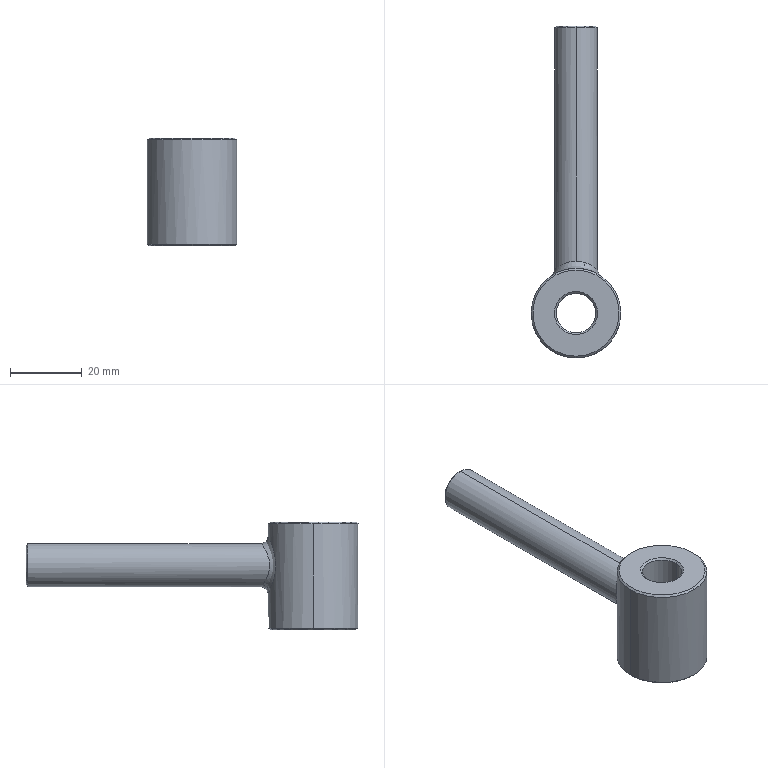Part | STEP file | M10-120_1 | 1 solid | 21 faces | box 25 x 92.5 x 30 mm | volume 19534 mm3 | cone 10 | cylinder 6 | plane 3 | spline 2 | commonest cylinder face diameters 11 x2 12 x2 25 x2